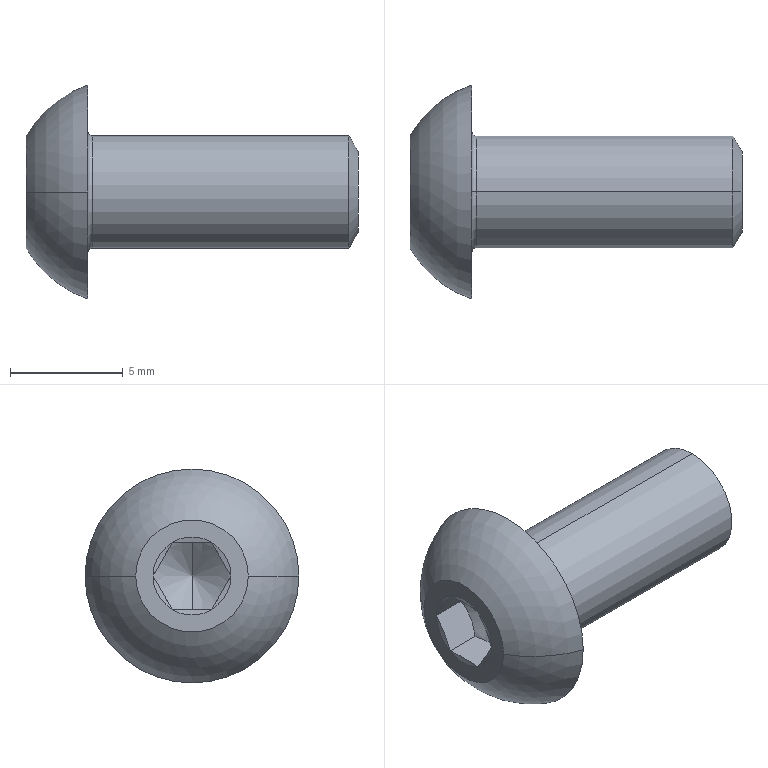Part | NX | features BREP 1 | 1 solid | 25 faces | box 14.75 x 9.5 x 9.5 mm | volume 353.31 mm3 | cone 10 | plane 9 | torus 2 | sphere 2 | cylinder 2 | commonest cylinder face diameters 5 x2
STEP:
#1=CARTESIAN_POINT('',(0.,0.,1.807));
#2=VERTEX_POINT('',#1);
#3=CARTESIAN_POINT('',(0.,0.,-1.807));
#4=VERTEX_POINT('',#3);
#5=CARTESIAN_POINT('',(0.,0.,0.));
#6=DIRECTION('',(-1.,0.,0.));
#7=DIRECTION('',(0.,0.,1.));
#8=AXIS2_PLACEMENT_3D('',#5,#6,#7);
#9=CIRCLE('',#8,1.807);
#10=EDGE_CURVE('',#2,#4,#9,.T.);
#11=ORIENTED_EDGE('',*,*,#10,.T.);
#12=CARTESIAN_POINT('',(-0.4,0.,-2.5));
#13=VERTEX_POINT('',#12);
#14=CARTESIAN_POINT('',(-0.4,0.,-2.5));
#15=DIRECTION('',(-0.5,0.,-0.866));
#16=VECTOR('',#15,1000.);
#17=LINE('',#14,#16);
#18=EDGE_CURVE('',#13,#4,#17,.F.);
#19=ORIENTED_EDGE('',*,*,#18,.F.);
#20=CARTESIAN_POINT('',(-0.4,0.,2.5));
#21=VERTEX_POINT('',#20);
#22=CARTESIAN_POINT('',(-0.4,0.,0.));
#23=DIRECTION('',(-1.,0.,0.));
#24=DIRECTION('',(0.,0.,1.));
#25=AXIS2_PLACEMENT_3D('',#22,#23,#24);
#26=CIRCLE('',#25,2.5);
#27=EDGE_CURVE('',#21,#13,#26,.T.);
#28=ORIENTED_EDGE('',*,*,#27,.F.);
#29=CARTESIAN_POINT('',(-0.4,0.,2.5));
#30=DIRECTION('',(-0.5,0.,0.866));
#31=VECTOR('',#30,1000.);
#32=LINE('',#29,#31);
#33=EDGE_CURVE('',#21,#2,#32,.F.);
#34=ORIENTED_EDGE('',*,*,#33,.T.);
#35=EDGE_LOOP('',(#11,#19,#28,#34));
#36=FACE_BOUND('',#35,.T.);
#37=CARTESIAN_POINT('',(-0.4,0.,0.));
#38=DIRECTION('',(-1.,0.,0.));
#39=DIRECTION('',(0.,0.,1.));
#40=AXIS2_PLACEMENT_3D('',#37,#38,#39);
#41=CONICAL_SURFACE('',#40,2.5,1.047);
#42=ADVANCED_FACE('',(#36),#41,.T.);
#43=CARTESIAN_POINT('',(-13.031,0.,1.5));
#44=VERTEX_POINT('',#43);
#45=CARTESIAN_POINT('',(-12.,0.,0.));
#46=VERTEX_POINT('',#45);
#47=CARTESIAN_POINT('',(-13.19,0.,1.732));
#48=DIRECTION('',(-0.5663,0.,0.8242));
#49=VECTOR('',#48,1000.);
#50=LINE('',#47,#49);
#51=EDGE_CURVE('',#44,#46,#50,.F.);
#52=ORIENTED_EDGE('',*,*,#51,.T.);
#53=CARTESIAN_POINT('',(-13.031,0.,-1.5));
#54=VERTEX_POINT('',#53);
#55=CARTESIAN_POINT('',(-13.19,0.,-1.732));
#56=DIRECTION('',(-0.5663,0.,-0.8242));
#57=VECTOR('',#56,1000.);
#58=LINE('',#55,#57);
#59=EDGE_CURVE('',#54,#46,#58,.F.);
#60=ORIENTED_EDGE('',*,*,#59,.F.);
#61=CARTESIAN_POINT('',(-13.19,-0.866,-1.5));
#62=VERTEX_POINT('',#61);
#63=CARTESIAN_POINT('',(-13.19,-0.866,-1.5));
#64=CARTESIAN_POINT('',(-13.087,-0.5676,-1.5));
#65=CARTESIAN_POINT('',(-13.031,-0.2874,-1.5));
#66=CARTESIAN_POINT('',(-13.031,0.,-1.5));
#67=B_SPLINE_CURVE_WITH_KNOTS('',3,(#63,#64,#65,#66),.UNSPECIFIED.,.F.,.F.,(4,4),(0.,1.),.UNSPECIFIED.);
#68=EDGE_CURVE('',#54,#62,#67,.F.);
#69=ORIENTED_EDGE('',*,*,#68,.T.);
#70=CARTESIAN_POINT('',(-13.19,-1.732,0.));
#71=VERTEX_POINT('',#70);
#72=CARTESIAN_POINT('',(-13.19,-1.732,0.));
#73=CARTESIAN_POINT('',(-12.984,-1.433,-0.5184));
#74=CARTESIAN_POINT('',(-12.985,-1.164,-0.9837));
#75=CARTESIAN_POINT('',(-13.19,-0.866,-1.5));
#76=B_SPLINE_CURVE_WITH_KNOTS('',3,(#72,#73,#74,#75),.UNSPECIFIED.,.F.,.F.,(4,4),(0.,1.),.UNSPECIFIED.);
#77=EDGE_CURVE('',#62,#71,#76,.F.);
#78=ORIENTED_EDGE('',*,*,#77,.T.);
#79=CARTESIAN_POINT('',(-13.19,-0.866,1.5));
#80=VERTEX_POINT('',#79);
#81=CARTESIAN_POINT('',(-13.19,-0.866,1.5));
#82=CARTESIAN_POINT('',(-12.984,-1.165,0.9816));
#83=CARTESIAN_POINT('',(-12.985,-1.434,0.5163));
#84=CARTESIAN_POINT('',(-13.19,-1.732,0.));
#85=B_SPLINE_CURVE_WITH_KNOTS('',3,(#81,#82,#83,#84),.UNSPECIFIED.,.F.,.F.,(4,4),(0.,1.),.UNSPECIFIED.);
#86=EDGE_CURVE('',#71,#80,#85,.F.);
#87=ORIENTED_EDGE('',*,*,#86,.T.);
#88=CARTESIAN_POINT('',(-13.031,0.,1.5));
#89=CARTESIAN_POINT('',(-13.031,-0.2844,1.5));
#90=CARTESIAN_POINT('',(-13.086,-0.5642,1.5));
#91=CARTESIAN_POINT('',(-13.19,-0.866,1.5));
#92=B_SPLINE_CURVE_WITH_KNOTS('',3,(#88,#89,#90,#91),.UNSPECIFIED.,.F.,.F.,(4,4),(0.,1.),.UNSPECIFIED.);
#93=EDGE_CURVE('',#80,#44,#92,.F.);
#94=ORIENTED_EDGE('',*,*,#93,.T.);
#95=EDGE_LOOP('',(#52,#60,#69,#78,#87,#94));
#96=FACE_BOUND('',#95,.T.);
#97=CARTESIAN_POINT('',(-13.19,0.,0.));
#98=DIRECTION('',(-1.,0.,0.));
#99=DIRECTION('',(0.,0.,1.));
#100=AXIS2_PLACEMENT_3D('',#97,#98,#99);
#101=CONICAL_SURFACE('',#100,1.732,0.9688);
#102=ADVANCED_FACE('',(#96),#101,.F.);
#103=CARTESIAN_POINT('',(-12.,0.,-2.7));
#104=VERTEX_POINT('',#103);
#105=CARTESIAN_POINT('',(-12.,0.,2.7));
#106=VERTEX_POINT('',#105);
#107=CARTESIAN_POINT('',(-12.,0.,0.));
#108=DIRECTION('',(-1.,0.,0.));
#109=DIRECTION('',(0.,0.,1.));
#110=AXIS2_PLACEMENT_3D('',#107,#108,#109);
#111=CIRCLE('',#110,2.7);
#112=EDGE_CURVE('',#104,#106,#111,.T.);
#113=ORIENTED_EDGE('',*,*,#112,.F.);
#114=CARTESIAN_POINT('',(-11.8,0.,-2.5));
#115=VERTEX_POINT('',#114);
#116=CARTESIAN_POINT('',(-11.8,0.,-2.7));
#117=DIRECTION('',(0.,1.,0.));
#118=DIRECTION('',(0.,0.,1.));
#119=AXIS2_PLACEMENT_3D('',#116,#117,#118);
#120=CIRCLE('',#119,0.2);
#121=EDGE_CURVE('',#115,#104,#120,.F.);
#122=ORIENTED_EDGE('',*,*,#121,.F.);
#123=CARTESIAN_POINT('',(-11.8,0.,2.5));
#124=VERTEX_POINT('',#123);
#125=CARTESIAN_POINT('',(-11.8,0.,0.));
#126=DIRECTION('',(-1.,0.,0.));
#127=DIRECTION('',(0.,0.,1.));
#128=AXIS2_PLACEMENT_3D('',#125,#126,#127);
#129=CIRCLE('',#128,2.5);
#130=EDGE_CURVE('',#115,#124,#129,.T.);
#131=ORIENTED_EDGE('',*,*,#130,.T.);
#132=CARTESIAN_POINT('',(-11.8,0.,2.7));
#133=DIRECTION('',(0.,-1.,0.));
#134=DIRECTION('',(0.,0.,-1.));
#135=AXIS2_PLACEMENT_3D('',#132,#133,#134);
#136=CIRCLE('',#135,0.2);
#137=EDGE_CURVE('',#124,#106,#136,.F.);
#138=ORIENTED_EDGE('',*,*,#137,.T.);
#139=EDGE_LOOP('',(#113,#122,#131,#138));
#140=FACE_BOUND('',#139,.T.);
#141=CARTESIAN_POINT('',(-11.8,0.,0.));
#142=DIRECTION('',(-1.,0.,0.));
#143=DIRECTION('',(0.,0.,1.));
#144=AXIS2_PLACEMENT_3D('',#141,#142,#143);
#145=TOROIDAL_SURFACE('',#144,2.7,0.2);
#146=ADVANCED_FACE('',(#140),#145,.F.);
#147=CARTESIAN_POINT('',(-12.,4.75,0.));
#148=VERTEX_POINT('',#147);
#149=CARTESIAN_POINT('',(-12.,-4.75,0.));
#150=VERTEX_POINT('',#149);
#151=CARTESIAN_POINT('',(-12.,0.,0.));
#152=DIRECTION('',(-1.,0.,0.));
#153=DIRECTION('',(0.,0.,1.));
#154=AXIS2_PLACEMENT_3D('',#151,#152,#153);
#155=CIRCLE('',#154,4.75);
#156=EDGE_CURVE('',#148,#150,#155,.T.);
#157=ORIENTED_EDGE('',*,*,#156,.T.);
#158=CARTESIAN_POINT('',(-14.75,-2.5,0.));
#159=VERTEX_POINT('',#158);
#160=CARTESIAN_POINT('',(-10.409,0.,0.));
#161=DIRECTION('',(0.,0.,-1.));
#162=DIRECTION('',(0.,1.,0.));
#163=AXIS2_PLACEMENT_3D('',#160,#161,#162);
#164=CIRCLE('',#163,5.009);
#165=EDGE_CURVE('',#159,#150,#164,.F.);
#166=ORIENTED_EDGE('',*,*,#165,.F.);
#167=CARTESIAN_POINT('',(-14.75,2.5,0.));
#168=VERTEX_POINT('',#167);
#169=CARTESIAN_POINT('',(-14.75,0.,0.));
#170=DIRECTION('',(-1.,0.,0.));
#171=DIRECTION('',(0.,0.,1.));
#172=AXIS2_PLACEMENT_3D('',#169,#170,#171);
#173=CIRCLE('',#172,2.5);
#174=EDGE_CURVE('',#168,#159,#173,.T.);
#175=ORIENTED_EDGE('',*,*,#174,.F.);
#176=CARTESIAN_POINT('',(-10.409,0.,0.));
#177=DIRECTION('',(0.,0.,1.));
#178=DIRECTION('',(1.,0.,0.));
#179=AXIS2_PLACEMENT_3D('',#176,#177,#178);
#180=CIRCLE('',#179,5.009);
#181=EDGE_CURVE('',#168,#148,#180,.F.);
#182=ORIENTED_EDGE('',*,*,#181,.T.);
#183=EDGE_LOOP('',(#157,#166,#175,#182));
#184=FACE_BOUND('',#183,.T.);
#185=CARTESIAN_POINT('',(-10.409,0.,0.));
#186=DIRECTION('',(1.,0.,0.));
#187=DIRECTION('',(0.,1.,0.));
#188=AXIS2_PLACEMENT_3D('',#185,#186,#187);
#189=SPHERICAL_SURFACE('',#188,5.009);
#190=ADVANCED_FACE('',(#184),#189,.T.);
#191=ORIENTED_EDGE('',*,*,#27,.T.);
#192=CARTESIAN_POINT('',(-14.75,0.,-2.5));
#193=DIRECTION('',(-1.,0.,0.));
#194=VECTOR('',#193,1000.);
#195=LINE('',#192,#194);
#196=EDGE_CURVE('',#115,#13,#195,.F.);
#197=ORIENTED_EDGE('',*,*,#196,.F.);
#198=CARTESIAN_POINT('',(-11.8,0.,0.));
#199=DIRECTION('',(-1.,0.,0.));
#200=DIRECTION('',(0.,0.,1.));
#201=AXIS2_PLACEMENT_3D('',#198,#199,#200);
#202=CIRCLE('',#201,2.5);
#203=EDGE_CURVE('',#124,#115,#202,.T.);
#204=ORIENTED_EDGE('',*,*,#203,.F.);
#205=CARTESIAN_POINT('',(-14.75,0.,2.5));
#206=DIRECTION('',(-1.,0.,0.));
#207=VECTOR('',#206,1000.);
#208=LINE('',#205,#207);
#209=EDGE_CURVE('',#124,#21,#208,.F.);
#210=ORIENTED_EDGE('',*,*,#209,.T.);
#211=EDGE_LOOP('',(#191,#197,#204,#210));
#212=FACE_BOUND('',#211,.T.);
#213=CARTESIAN_POINT('',(-14.75,0.,0.));
#214=DIRECTION('',(-1.,0.,0.));
#215=DIRECTION('',(0.,0.,1.));
#216=AXIS2_PLACEMENT_3D('',#213,#214,#215);
#217=CYLINDRICAL_SURFACE('',#216,2.5);
#218=ADVANCED_FACE('',(#212),#217,.T.);
#219=ORIENTED_EDGE('',*,*,#196,.T.);
#220=CARTESIAN_POINT('',(-0.4,0.,0.));
#221=DIRECTION('',(-1.,0.,0.));
#222=DIRECTION('',(0.,0.,1.));
#223=AXIS2_PLACEMENT_3D('',#220,#221,#222);
#224=CIRCLE('',#223,2.5);
#225=EDGE_CURVE('',#13,#21,#224,.T.);
#226=ORIENTED_EDGE('',*,*,#225,.T.);
#227=ORIENTED_EDGE('',*,*,#209,.F.);
#228=ORIENTED_EDGE('',*,*,#130,.F.);
#229=EDGE_LOOP('',(#219,#226,#227,#228));
#230=FACE_BOUND('',#229,.T.);
#231=CARTESIAN_POINT('',(-14.75,0.,0.));
#232=DIRECTION('',(-1.,0.,0.));
#233=DIRECTION('',(0.,0.,1.));
#234=AXIS2_PLACEMENT_3D('',#231,#232,#233);
#235=CYLINDRICAL_SURFACE('',#234,2.5);
#236=ADVANCED_FACE('',(#230),#235,.T.);
#237=ORIENTED_EDGE('',*,*,#174,.T.);
#238=CARTESIAN_POINT('',(-14.75,0.,0.));
#239=DIRECTION('',(-1.,0.,0.));
#240=DIRECTION('',(0.,0.,1.));
#241=AXIS2_PLACEMENT_3D('',#238,#239,#240);
#242=CIRCLE('',#241,2.5);
#243=EDGE_CURVE('',#159,#168,#242,.T.);
#244=ORIENTED_EDGE('',*,*,#243,.T.);
#245=EDGE_LOOP('',(#237,#244));
#246=FACE_BOUND('',#245,.T.);
#247=CARTESIAN_POINT('',(-14.75,-0.866,-1.5));
#248=VERTEX_POINT('',#247);
#249=CARTESIAN_POINT('',(-14.75,-1.732,0.));
#250=VERTEX_POINT('',#249);
#251=CARTESIAN_POINT('',(-14.75,0.,0.));
#252=DIRECTION('',(-1.,0.,0.));
#253=DIRECTION('',(0.,0.,-1.));
#254=AXIS2_PLACEMENT_3D('',#251,#252,#253);
#255=CIRCLE('',#254,1.732);
#256=EDGE_CURVE('',#248,#250,#255,.T.);
#257=ORIENTED_EDGE('',*,*,#256,.F.);
#258=CARTESIAN_POINT('',(-14.75,0.866,-1.5));
#259=VERTEX_POINT('',#258);
#260=CARTESIAN_POINT('',(-14.75,0.,0.));
#261=DIRECTION('',(-1.,0.,0.));
#262=DIRECTION('',(0.,0.,-1.));
#263=AXIS2_PLACEMENT_3D('',#260,#261,#262);
#264=CIRCLE('',#263,1.732);
#265=EDGE_CURVE('',#259,#248,#264,.T.);
#266=ORIENTED_EDGE('',*,*,#265,.F.);
#267=CARTESIAN_POINT('',(-14.75,1.732,0.));
#268=VERTEX_POINT('',#267);
#269=CARTESIAN_POINT('',(-14.75,0.,0.));
#270=DIRECTION('',(-1.,0.,0.));
#271=DIRECTION('',(0.,0.,-1.));
#272=AXIS2_PLACEMENT_3D('',#269,#270,#271);
#273=CIRCLE('',#272,1.732);
#274=EDGE_CURVE('',#268,#259,#273,.T.);
#275=ORIENTED_EDGE('',*,*,#274,.F.);
#276=CARTESIAN_POINT('',(-14.75,0.866,1.5));
#277=VERTEX_POINT('',#276);
#278=CARTESIAN_POINT('',(-14.75,0.,0.));
#279=DIRECTION('',(-1.,0.,0.));
#280=DIRECTION('',(0.,0.,-1.));
#281=AXIS2_PLACEMENT_3D('',#278,#279,#280);
#282=CIRCLE('',#281,1.732);
#283=EDGE_CURVE('',#277,#268,#282,.T.);
#284=ORIENTED_EDGE('',*,*,#283,.F.);
#285=CARTESIAN_POINT('',(-14.75,-0.866,1.5));
#286=VERTEX_POINT('',#285);
#287=CARTESIAN_POINT('',(-14.75,0.,0.));
#288=DIRECTION('',(-1.,0.,0.));
#289=DIRECTION('',(0.,0.,-1.));
#290=AXIS2_PLACEMENT_3D('',#287,#288,#289);
#291=CIRCLE('',#290,1.732);
#292=EDGE_CURVE('',#286,#277,#291,.T.);
#293=ORIENTED_EDGE('',*,*,#292,.F.);
#294=CARTESIAN_POINT('',(-14.75,0.,0.));
#295=DIRECTION('',(-1.,0.,0.));
#296=DIRECTION('',(0.,-1.,0.));
#297=AXIS2_PLACEMENT_3D('',#294,#295,#296);
#298=CIRCLE('',#297,1.732);
#299=EDGE_CURVE('',#250,#286,#298,.T.);
#300=ORIENTED_EDGE('',*,*,#299,.F.);
#301=EDGE_LOOP('',(#257,#266,#275,#284,#293,#300));
#302=FACE_BOUND('',#301,.T.);
#303=CARTESIAN_POINT('',(-14.75,0.,0.));
#304=DIRECTION('',(1.,0.,0.));
#305=DIRECTION('',(0.,1.,0.));
#306=AXIS2_PLACEMENT_3D('',#303,#304,#305);
#307=PLANE('',#306);
#308=ADVANCED_FACE('',(#246,#302),#307,.F.);
#309=ORIENTED_EDGE('',*,*,#165,.T.);
#310=CARTESIAN_POINT('',(-12.,0.,0.));
#311=DIRECTION('',(-1.,0.,0.));
#312=DIRECTION('',(0.,0.,1.));
#313=AXIS2_PLACEMENT_3D('',#310,#311,#312);
#314=CIRCLE('',#313,4.75);
#315=EDGE_CURVE('',#150,#148,#314,.T.);
#316=ORIENTED_EDGE('',*,*,#315,.T.);
#317=ORIENTED_EDGE('',*,*,#181,.F.);
#318=ORIENTED_EDGE('',*,*,#243,.F.);
#319=EDGE_LOOP('',(#309,#316,#317,#318));
#320=FACE_BOUND('',#319,.T.);
#321=CARTESIAN_POINT('',(-10.409,0.,0.));
#322=DIRECTION('',(1.,0.,0.));
#323=DIRECTION('',(0.,1.,0.));
#324=AXIS2_PLACEMENT_3D('',#321,#322,#323);
#325=SPHERICAL_SURFACE('',#324,5.009);
#326=ADVANCED_FACE('',(#320),#325,.T.);
#327=ORIENTED_EDGE('',*,*,#156,.F.);
#328=ORIENTED_EDGE('',*,*,#315,.F.);
#329=EDGE_LOOP('',(#327,#328));
#330=FACE_BOUND('',#329,.T.);
#331=CARTESIAN_POINT('',(-12.,0.,0.));
#332=DIRECTION('',(-1.,0.,0.));
#333=DIRECTION('',(0.,0.,1.));
#334=AXIS2_PLACEMENT_3D('',#331,#332,#333);
#335=CIRCLE('',#334,2.7);
#336=EDGE_CURVE('',#106,#104,#335,.T.);
#337=ORIENTED_EDGE('',*,*,#336,.T.);
#338=ORIENTED_EDGE('',*,*,#112,.T.);
#339=EDGE_LOOP('',(#337,#338));
#340=FACE_BOUND('',#339,.T.);
#341=CARTESIAN_POINT('',(-12.,2.7,0.));
#342=DIRECTION('',(-1.,0.,0.));
#343=DIRECTION('',(0.,0.,1.));
#344=AXIS2_PLACEMENT_3D('',#341,#342,#343);
#345=PLANE('',#344);
#346=ADVANCED_FACE('',(#330,#340),#345,.F.);
#347=ORIENTED_EDGE('',*,*,#121,.T.);
#348=ORIENTED_EDGE('',*,*,#336,.F.);
#349=ORIENTED_EDGE('',*,*,#137,.F.);
#350=ORIENTED_EDGE('',*,*,#203,.T.);
#351=EDGE_LOOP('',(#347,#348,#349,#350));
#352=FACE_BOUND('',#351,.T.);
#353=CARTESIAN_POINT('',(-11.8,0.,0.));
#354=DIRECTION('',(-1.,0.,0.));
#355=DIRECTION('',(0.,0.,1.));
#356=AXIS2_PLACEMENT_3D('',#353,#354,#355);
#357=TOROIDAL_SURFACE('',#356,2.7,0.2);
#358=ADVANCED_FACE('',(#352),#357,.F.);
#359=CARTESIAN_POINT('',(-14.75,0.866,-1.5));
#360=CARTESIAN_POINT('',(-14.672,0.2486,-1.5));
#361=CARTESIAN_POINT('',(-14.671,-0.2459,-1.5));
#362=CARTESIAN_POINT('',(-14.75,-0.866,-1.5));
#363=B_SPLINE_CURVE_WITH_KNOTS('',3,(#359,#360,#361,#362),.UNSPECIFIED.,.F.,.F.,(4,4),(0.,1.),.UNSPECIFIED.);
#364=EDGE_CURVE('',#248,#259,#363,.F.);
#365=ORIENTED_EDGE('',*,*,#364,.T.);
#366=ORIENTED_EDGE('',*,*,#265,.T.);
#367=EDGE_LOOP('',(#365,#366));
#368=FACE_BOUND('',#367,.T.);
#369=CARTESIAN_POINT('',(-1014.31,0.,0.));
#370=DIRECTION('',(-1.,0.,0.));
#371=DIRECTION('',(0.,-1.,0.));
#372=AXIS2_PLACEMENT_3D('',#369,#370,#371);
#373=CONICAL_SURFACE('',#372,3936.479,1.322);
#374=ADVANCED_FACE('',(#368),#373,.F.);
#375=CARTESIAN_POINT('',(-14.75,1.732,0.));
#376=CARTESIAN_POINT('',(-14.671,1.423,-0.5356));
#377=CARTESIAN_POINT('',(-14.671,1.176,-0.9638));
#378=CARTESIAN_POINT('',(-14.75,0.866,-1.5));
#379=B_SPLINE_CURVE_WITH_KNOTS('',3,(#375,#376,#377,#378),.UNSPECIFIED.,.F.,.F.,(4,4),(0.,1.),.UNSPECIFIED.);
#380=EDGE_CURVE('',#259,#268,#379,.F.);
#381=ORIENTED_EDGE('',*,*,#380,.T.);
#382=ORIENTED_EDGE('',*,*,#274,.T.);
#383=EDGE_LOOP('',(#381,#382));
#384=FACE_BOUND('',#383,.T.);
#385=CARTESIAN_POINT('',(-1014.31,0.,0.));
#386=DIRECTION('',(-1.,0.,0.));
#387=DIRECTION('',(0.,-1.,0.));
#388=AXIS2_PLACEMENT_3D('',#385,#386,#387);
#389=CONICAL_SURFACE('',#388,3936.479,1.322);
#390=ADVANCED_FACE('',(#384),#389,.F.);
#391=CARTESIAN_POINT('',(-14.75,0.866,1.5));
#392=CARTESIAN_POINT('',(-14.671,1.175,0.9644));
#393=CARTESIAN_POINT('',(-14.671,1.422,0.5362));
#394=CARTESIAN_POINT('',(-14.75,1.732,0.));
#395=B_SPLINE_CURVE_WITH_KNOTS('',3,(#391,#392,#393,#394),.UNSPECIFIED.,.F.,.F.,(4,4),(0.,1.),.UNSPECIFIED.);
#396=EDGE_CURVE('',#268,#277,#395,.F.);
#397=ORIENTED_EDGE('',*,*,#396,.T.);
#398=ORIENTED_EDGE('',*,*,#283,.T.);
#399=EDGE_LOOP('',(#397,#398));
#400=FACE_BOUND('',#399,.T.);
#401=CARTESIAN_POINT('',(-1014.31,0.,0.));
#402=DIRECTION('',(-1.,0.,0.));
#403=DIRECTION('',(0.,-1.,0.));
#404=AXIS2_PLACEMENT_3D('',#401,#402,#403);
#405=CONICAL_SURFACE('',#404,3936.479,1.322);
#406=ADVANCED_FACE('',(#400),#405,.F.);
#407=CARTESIAN_POINT('',(-14.75,-0.866,1.5));
#408=CARTESIAN_POINT('',(-14.671,-0.2465,1.5));
#409=CARTESIAN_POINT('',(-14.671,0.2479,1.5));
#410=CARTESIAN_POINT('',(-14.75,0.866,1.5));
#411=B_SPLINE_CURVE_WITH_KNOTS('',3,(#407,#408,#409,#410),.UNSPECIFIED.,.F.,.F.,(4,4),(0.,1.),.UNSPECIFIED.);
#412=EDGE_CURVE('',#277,#286,#411,.F.);
#413=ORIENTED_EDGE('',*,*,#412,.T.);
#414=ORIENTED_EDGE('',*,*,#292,.T.);
#415=EDGE_LOOP('',(#413,#414));
#416=FACE_BOUND('',#415,.T.);
#417=CARTESIAN_POINT('',(-1014.31,0.,0.));
#418=DIRECTION('',(-1.,0.,0.));
#419=DIRECTION('',(0.,-1.,0.));
#420=AXIS2_PLACEMENT_3D('',#417,#418,#419);
#421=CONICAL_SURFACE('',#420,3936.479,1.322);
#422=ADVANCED_FACE('',(#416),#421,.F.);
#423=CARTESIAN_POINT('',(-14.75,-1.732,0.));
#424=CARTESIAN_POINT('',(-14.671,-1.423,0.5356));
#425=CARTESIAN_POINT('',(-14.671,-1.176,0.9638));
#426=CARTESIAN_POINT('',(-14.75,-0.866,1.5));
#427=B_SPLINE_CURVE_WITH_KNOTS('',3,(#423,#424,#425,#426),.UNSPECIFIED.,.F.,.F.,(4,4),(0.,1.),.UNSPECIFIED.);
#428=EDGE_CURVE('',#286,#250,#427,.F.);
#429=ORIENTED_EDGE('',*,*,#428,.T.);
#430=ORIENTED_EDGE('',*,*,#299,.T.);
#431=EDGE_LOOP('',(#429,#430));
#432=FACE_BOUND('',#431,.T.);
#433=CARTESIAN_POINT('',(-1014.31,0.,0.));
#434=DIRECTION('',(-1.,0.,0.));
#435=DIRECTION('',(0.,-1.,0.));
#436=AXIS2_PLACEMENT_3D('',#433,#434,#435);
#437=CONICAL_SURFACE('',#436,3936.479,1.322);
#438=ADVANCED_FACE('',(#432),#437,.F.);
#439=CARTESIAN_POINT('',(-14.75,-0.866,-1.5));
#440=CARTESIAN_POINT('',(-14.671,-1.175,-0.9644));
#441=CARTESIAN_POINT('',(-14.671,-1.422,-0.5362));
#442=CARTESIAN_POINT('',(-14.75,-1.732,0.));
#443=B_SPLINE_CURVE_WITH_KNOTS('',3,(#439,#440,#441,#442),.UNSPECIFIED.,.F.,.F.,(4,4),(0.,1.),.UNSPECIFIED.);
#444=EDGE_CURVE('',#250,#248,#443,.F.);
#445=ORIENTED_EDGE('',*,*,#444,.T.);
#446=ORIENTED_EDGE('',*,*,#256,.T.);
#447=EDGE_LOOP('',(#445,#446));
#448=FACE_BOUND('',#447,.T.);
#449=CARTESIAN_POINT('',(-1014.31,0.,0.));
#450=DIRECTION('',(-1.,0.,0.));
#451=DIRECTION('',(0.,-1.,0.));
#452=AXIS2_PLACEMENT_3D('',#449,#450,#451);
#453=CONICAL_SURFACE('',#452,3936.479,1.322);
#454=ADVANCED_FACE('',(#448),#453,.F.);
#455=ORIENTED_EDGE('',*,*,#59,.T.);
#456=ORIENTED_EDGE('',*,*,#51,.F.);
#457=CARTESIAN_POINT('',(-13.19,0.866,1.5));
#458=VERTEX_POINT('',#457);
#459=CARTESIAN_POINT('',(-13.19,0.866,1.5));
#460=CARTESIAN_POINT('',(-13.088,0.5699,1.5));
#461=CARTESIAN_POINT('',(-13.031,0.2894,1.5));
#462=CARTESIAN_POINT('',(-13.031,0.,1.5));
#463=B_SPLINE_CURVE_WITH_KNOTS('',3,(#459,#460,#461,#462),.UNSPECIFIED.,.F.,.F.,(4,4),(0.,1.),.UNSPECIFIED.);
#464=EDGE_CURVE('',#44,#458,#463,.F.);
#465=ORIENTED_EDGE('',*,*,#464,.T.);
#466=CARTESIAN_POINT('',(-13.19,1.732,0.));
#467=VERTEX_POINT('',#466);
#468=CARTESIAN_POINT('',(-13.19,1.732,0.));
#469=CARTESIAN_POINT('',(-12.984,1.433,0.5184));
#470=CARTESIAN_POINT('',(-12.985,1.164,0.9837));
#471=CARTESIAN_POINT('',(-13.19,0.866,1.5));
#472=B_SPLINE_CURVE_WITH_KNOTS('',3,(#468,#469,#470,#471),.UNSPECIFIED.,.F.,.F.,(4,4),(0.,1.),.UNSPECIFIED.);
#473=EDGE_CURVE('',#458,#467,#472,.F.);
#474=ORIENTED_EDGE('',*,*,#473,.T.);
#475=CARTESIAN_POINT('',(-13.19,0.866,-1.5));
#476=VERTEX_POINT('',#475);
#477=CARTESIAN_POINT('',(-13.19,0.866,-1.5));
#478=CARTESIAN_POINT('',(-12.984,1.165,-0.9816));
#479=CARTESIAN_POINT('',(-12.985,1.434,-0.5163));
#480=CARTESIAN_POINT('',(-13.19,1.732,0.));
#481=B_SPLINE_CURVE_WITH_KNOTS('',3,(#477,#478,#479,#480),.UNSPECIFIED.,.F.,.F.,(4,4),(0.,1.),.UNSPECIFIED.);
#482=EDGE_CURVE('',#467,#476,#481,.F.);
#483=ORIENTED_EDGE('',*,*,#482,.T.);
#484=CARTESIAN_POINT('',(-13.031,0.,-1.5));
#485=CARTESIAN_POINT('',(-13.031,0.2864,-1.5));
#486=CARTESIAN_POINT('',(-13.087,0.5665,-1.5));
#487=CARTESIAN_POINT('',(-13.19,0.866,-1.5));
#488=B_SPLINE_CURVE_WITH_KNOTS('',3,(#484,#485,#486,#487),.UNSPECIFIED.,.F.,.F.,(4,4),(0.,1.),.UNSPECIFIED.);
#489=EDGE_CURVE('',#476,#54,#488,.F.);
#490=ORIENTED_EDGE('',*,*,#489,.T.);
#491=EDGE_LOOP('',(#455,#456,#465,#474,#483,#490));
#492=FACE_BOUND('',#491,.T.);
#493=CARTESIAN_POINT('',(-13.19,0.,0.));
#494=DIRECTION('',(-1.,0.,0.));
#495=DIRECTION('',(0.,0.,1.));
#496=AXIS2_PLACEMENT_3D('',#493,#494,#495);
#497=CONICAL_SURFACE('',#496,1.732,0.9688);
#498=ADVANCED_FACE('',(#492),#497,.F.);
#499=ORIENTED_EDGE('',*,*,#380,.F.);
#500=CARTESIAN_POINT('',(-12.,0.866,-1.5));
#501=DIRECTION('',(-1.,0.,0.));
#502=VECTOR('',#501,1000.);
#503=LINE('',#500,#502);
#504=EDGE_CURVE('',#476,#259,#503,.T.);
#505=ORIENTED_EDGE('',*,*,#504,.F.);
#506=ORIENTED_EDGE('',*,*,#482,.F.);
#507=CARTESIAN_POINT('',(-12.,1.732,0.));
#508=DIRECTION('',(-1.,0.,0.));
#509=VECTOR('',#508,1000.);
#510=LINE('',#507,#509);
#511=EDGE_CURVE('',#467,#268,#510,.T.);
#512=ORIENTED_EDGE('',*,*,#511,.T.);
#513=EDGE_LOOP('',(#499,#505,#506,#512));
#514=FACE_BOUND('',#513,.T.);
#515=CARTESIAN_POINT('',(-12.,1.732,0.));
#516=DIRECTION('',(0.,0.866,-0.5));
#517=DIRECTION('',(-1.,0.,0.));
#518=AXIS2_PLACEMENT_3D('',#515,#516,#517);
#519=PLANE('',#518);
#520=ADVANCED_FACE('',(#514),#519,.F.);
#521=ORIENTED_EDGE('',*,*,#364,.F.);
#522=CARTESIAN_POINT('',(-12.,-0.866,-1.5));
#523=DIRECTION('',(-1.,0.,0.));
#524=VECTOR('',#523,1000.);
#525=LINE('',#522,#524);
#526=EDGE_CURVE('',#62,#248,#525,.T.);
#527=ORIENTED_EDGE('',*,*,#526,.F.);
#528=ORIENTED_EDGE('',*,*,#68,.F.);
#529=ORIENTED_EDGE('',*,*,#489,.F.);
#530=ORIENTED_EDGE('',*,*,#504,.T.);
#531=EDGE_LOOP('',(#521,#527,#528,#529,#530));
#532=FACE_BOUND('',#531,.T.);
#533=CARTESIAN_POINT('',(-12.,0.866,-1.5));
#534=DIRECTION('',(0.,0.,-1.));
#535=DIRECTION('',(0.,-1.,0.));
#536=AXIS2_PLACEMENT_3D('',#533,#534,#535);
#537=PLANE('',#536);
#538=ADVANCED_FACE('',(#532),#537,.F.);
#539=ORIENTED_EDGE('',*,*,#444,.F.);
#540=CARTESIAN_POINT('',(-12.,-1.732,0.));
#541=DIRECTION('',(-1.,0.,0.));
#542=VECTOR('',#541,1000.);
#543=LINE('',#540,#542);
#544=EDGE_CURVE('',#71,#250,#543,.T.);
#545=ORIENTED_EDGE('',*,*,#544,.F.);
#546=ORIENTED_EDGE('',*,*,#77,.F.);
#547=ORIENTED_EDGE('',*,*,#526,.T.);
#548=EDGE_LOOP('',(#539,#545,#546,#547));
#549=FACE_BOUND('',#548,.T.);
#550=CARTESIAN_POINT('',(-12.,-0.866,-1.5));
#551=DIRECTION('',(0.,-0.866,-0.5));
#552=DIRECTION('',(0.,0.5,-0.866));
#553=AXIS2_PLACEMENT_3D('',#550,#551,#552);
#554=PLANE('',#553);
#555=ADVANCED_FACE('',(#549),#554,.F.);
#556=ORIENTED_EDGE('',*,*,#428,.F.);
#557=CARTESIAN_POINT('',(-12.,-0.866,1.5));
#558=DIRECTION('',(-1.,0.,0.));
#559=VECTOR('',#558,1000.);
#560=LINE('',#557,#559);
#561=EDGE_CURVE('',#80,#286,#560,.T.);
#562=ORIENTED_EDGE('',*,*,#561,.F.);
#563=ORIENTED_EDGE('',*,*,#86,.F.);
#564=ORIENTED_EDGE('',*,*,#544,.T.);
#565=EDGE_LOOP('',(#556,#562,#563,#564));
#566=FACE_BOUND('',#565,.T.);
#567=CARTESIAN_POINT('',(-12.,-1.732,0.));
#568=DIRECTION('',(0.,-0.866,0.5));
#569=DIRECTION('',(-1.,0.,0.));
#570=AXIS2_PLACEMENT_3D('',#567,#568,#569);
#571=PLANE('',#570);
#572=ADVANCED_FACE('',(#566),#571,.F.);
#573=ORIENTED_EDGE('',*,*,#412,.F.);
#574=CARTESIAN_POINT('',(-12.,0.866,1.5));
#575=DIRECTION('',(-1.,0.,0.));
#576=VECTOR('',#575,1000.);
#577=LINE('',#574,#576);
#578=EDGE_CURVE('',#458,#277,#577,.T.);
#579=ORIENTED_EDGE('',*,*,#578,.F.);
#580=ORIENTED_EDGE('',*,*,#464,.F.);
#581=ORIENTED_EDGE('',*,*,#93,.F.);
#582=ORIENTED_EDGE('',*,*,#561,.T.);
#583=EDGE_LOOP('',(#573,#579,#580,#581,#582));
#584=FACE_BOUND('',#583,.T.);
#585=CARTESIAN_POINT('',(-12.,-0.866,1.5));
#586=DIRECTION('',(0.,0.,1.));
#587=DIRECTION('',(1.,0.,0.));
#588=AXIS2_PLACEMENT_3D('',#585,#586,#587);
#589=PLANE('',#588);
#590=ADVANCED_FACE('',(#584),#589,.F.);
#591=ORIENTED_EDGE('',*,*,#396,.F.);
#592=ORIENTED_EDGE('',*,*,#511,.F.);
#593=ORIENTED_EDGE('',*,*,#473,.F.);
#594=ORIENTED_EDGE('',*,*,#578,.T.);
#595=EDGE_LOOP('',(#591,#592,#593,#594));
#596=FACE_BOUND('',#595,.T.);
#597=CARTESIAN_POINT('',(-12.,0.866,1.5));
#598=DIRECTION('',(0.,0.866,0.5));
#599=DIRECTION('',(1.,0.,0.));
#600=AXIS2_PLACEMENT_3D('',#597,#598,#599);
#601=PLANE('',#600);
#602=ADVANCED_FACE('',(#596),#601,.F.);
#603=ORIENTED_EDGE('',*,*,#18,.T.);
#604=CARTESIAN_POINT('',(0.,0.,0.));
#605=DIRECTION('',(-1.,0.,0.));
#606=DIRECTION('',(0.,0.,1.));
#607=AXIS2_PLACEMENT_3D('',#604,#605,#606);
#608=CIRCLE('',#607,1.807);
#609=EDGE_CURVE('',#4,#2,#608,.T.);
#610=ORIENTED_EDGE('',*,*,#609,.T.);
#611=ORIENTED_EDGE('',*,*,#33,.F.);
#612=ORIENTED_EDGE('',*,*,#225,.F.);
#613=EDGE_LOOP('',(#603,#610,#611,#612));
#614=FACE_BOUND('',#613,.T.);
#615=CARTESIAN_POINT('',(-0.4,0.,0.));
#616=DIRECTION('',(-1.,0.,0.));
#617=DIRECTION('',(0.,0.,1.));
#618=AXIS2_PLACEMENT_3D('',#615,#616,#617);
#619=CONICAL_SURFACE('',#618,2.5,1.047);
#620=ADVANCED_FACE('',(#614),#619,.T.);
#621=ORIENTED_EDGE('',*,*,#10,.F.);
#622=ORIENTED_EDGE('',*,*,#609,.F.);
#623=EDGE_LOOP('',(#621,#622));
#624=FACE_BOUND('',#623,.T.);
#625=CARTESIAN_POINT('',(0.,2.5,0.));
#626=DIRECTION('',(-1.,0.,0.));
#627=DIRECTION('',(0.,0.,1.));
#628=AXIS2_PLACEMENT_3D('',#625,#626,#627);
#629=PLANE('',#628);
#630=ADVANCED_FACE('',(#624),#629,.F.);
#631=CLOSED_SHELL('',(#42,#102,#146,#190,#218,#236,#308,#326,#346,#358,#374,#390,#406,#422,#438,#454,#498,#520,#538,#555,#572,#590,#602,#620,#630));
#632=MANIFOLD_SOLID_BREP('',#631);
#633=(LENGTH_UNIT()NAMED_UNIT(*)SI_UNIT(.MILLI.,.METRE.));
#634=UNCERTAINTY_MEASURE_WITH_UNIT(LENGTH_MEASURE(0.0508),#633,'','');
#635=(NAMED_UNIT(*)PLANE_ANGLE_UNIT()SI_UNIT($,.RADIAN.));
#636=(NAMED_UNIT(*)SI_UNIT($,.STERADIAN.)SOLID_ANGLE_UNIT());
#637=(GEOMETRIC_REPRESENTATION_CONTEXT(3)GLOBAL_UNCERTAINTY_ASSIGNED_CONTEXT((#634))GLOBAL_UNIT_ASSIGNED_CONTEXT((#633,#635,#636))REPRESENTATION_CONTEXT('',''));
#638=ADVANCED_BREP_SHAPE_REPRESENTATION('',(#632),#637);